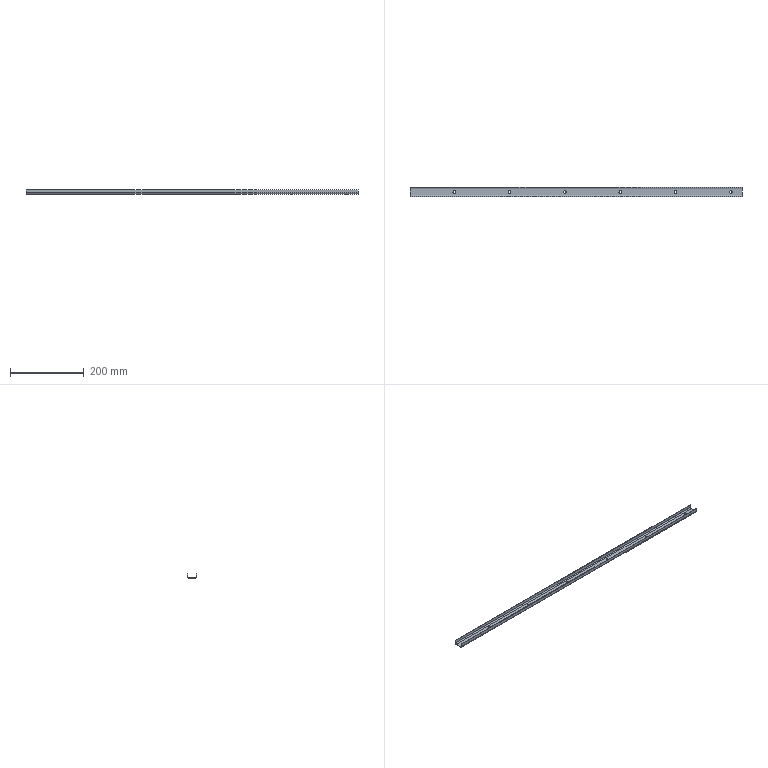Part | NX | features SKETCH 4, DATUM_CSYS 3, DATUM_PLANE 2, Flange 2, Base Tab 1, EXTRUDE 1 | 1 solid | 20 faces | box 900 x 25 x 12 mm | volume 46713 mm3 | plane 10 | cylinder 10 | commonest cylinder face diameters 7 x6 6 x2 8.4 x2
STEP:
#1=CARTESIAN_POINT('',(0.,20.8,0.));
#2=VERTEX_POINT('',#1);
#3=CARTESIAN_POINT('',(0.,4.2,0.));
#4=VERTEX_POINT('',#3);
#5=CARTESIAN_POINT('',(0.,25.,0.));
#6=DIRECTION('',(0.,-1.,0.));
#7=VECTOR('',#6,1000.);
#8=LINE('',#5,#7);
#9=EDGE_CURVE('',#2,#4,#8,.T.);
#10=ORIENTED_EDGE('',*,*,#9,.T.);
#11=CARTESIAN_POINT('',(0.,0.,4.2));
#12=VERTEX_POINT('',#11);
#13=CARTESIAN_POINT('',(0.,4.2,4.2));
#14=DIRECTION('',(-1.,0.,0.));
#15=DIRECTION('',(0.,0.,1.));
#16=AXIS2_PLACEMENT_3D('',#13,#14,#15);
#17=CIRCLE('',#16,4.2);
#18=EDGE_CURVE('',#4,#12,#17,.T.);
#19=ORIENTED_EDGE('',*,*,#18,.T.);
#20=CARTESIAN_POINT('',(0.,0.,12.));
#21=VERTEX_POINT('',#20);
#22=CARTESIAN_POINT('',(0.,0.,1.533));
#23=DIRECTION('',(0.,0.,1.));
#24=VECTOR('',#23,1000.);
#25=LINE('',#22,#24);
#26=EDGE_CURVE('',#12,#21,#25,.T.);
#27=ORIENTED_EDGE('',*,*,#26,.T.);
#28=CARTESIAN_POINT('',(0.,1.2,12.));
#29=VERTEX_POINT('',#28);
#30=CARTESIAN_POINT('',(0.,0.,12.));
#31=DIRECTION('',(0.,1.,0.));
#32=VECTOR('',#31,1000.);
#33=LINE('',#30,#32);
#34=EDGE_CURVE('',#21,#29,#33,.T.);
#35=ORIENTED_EDGE('',*,*,#34,.T.);
#36=CARTESIAN_POINT('',(0.,1.2,4.2));
#37=VERTEX_POINT('',#36);
#38=CARTESIAN_POINT('',(0.,1.2,1.533));
#39=DIRECTION('',(0.,0.,1.));
#40=VECTOR('',#39,1000.);
#41=LINE('',#38,#40);
#42=EDGE_CURVE('',#37,#29,#41,.T.);
#43=ORIENTED_EDGE('',*,*,#42,.F.);
#44=CARTESIAN_POINT('',(0.,4.2,1.2));
#45=VERTEX_POINT('',#44);
#46=CARTESIAN_POINT('',(0.,4.2,4.2));
#47=DIRECTION('',(-1.,0.,0.));
#48=DIRECTION('',(0.,0.,1.));
#49=AXIS2_PLACEMENT_3D('',#46,#47,#48);
#50=CIRCLE('',#49,3.);
#51=EDGE_CURVE('',#45,#37,#50,.T.);
#52=ORIENTED_EDGE('',*,*,#51,.F.);
#53=CARTESIAN_POINT('',(0.,20.8,1.2));
#54=VERTEX_POINT('',#53);
#55=CARTESIAN_POINT('',(0.,25.,1.2));
#56=DIRECTION('',(0.,-1.,0.));
#57=VECTOR('',#56,1000.);
#58=LINE('',#55,#57);
#59=EDGE_CURVE('',#54,#45,#58,.T.);
#60=ORIENTED_EDGE('',*,*,#59,.F.);
#61=CARTESIAN_POINT('',(0.,23.8,4.2));
#62=VERTEX_POINT('',#61);
#63=CARTESIAN_POINT('',(0.,20.8,4.2));
#64=DIRECTION('',(1.,0.,0.));
#65=DIRECTION('',(0.,0.,-1.));
#66=AXIS2_PLACEMENT_3D('',#63,#64,#65);
#67=CIRCLE('',#66,3.);
#68=EDGE_CURVE('',#62,#54,#67,.F.);
#69=ORIENTED_EDGE('',*,*,#68,.F.);
#70=CARTESIAN_POINT('',(0.,23.8,12.));
#71=VERTEX_POINT('',#70);
#72=CARTESIAN_POINT('',(0.,23.8,1.533));
#73=DIRECTION('',(0.,0.,1.));
#74=VECTOR('',#73,1000.);
#75=LINE('',#72,#74);
#76=EDGE_CURVE('',#62,#71,#75,.T.);
#77=ORIENTED_EDGE('',*,*,#76,.T.);
#78=CARTESIAN_POINT('',(0.,25.,12.));
#79=VERTEX_POINT('',#78);
#80=CARTESIAN_POINT('',(0.,25.,12.));
#81=DIRECTION('',(0.,-1.,0.));
#82=VECTOR('',#81,1000.);
#83=LINE('',#80,#82);
#84=EDGE_CURVE('',#79,#71,#83,.T.);
#85=ORIENTED_EDGE('',*,*,#84,.F.);
#86=CARTESIAN_POINT('',(0.,25.,4.2));
#87=VERTEX_POINT('',#86);
#88=CARTESIAN_POINT('',(0.,25.,1.533));
#89=DIRECTION('',(0.,0.,1.));
#90=VECTOR('',#89,1000.);
#91=LINE('',#88,#90);
#92=EDGE_CURVE('',#87,#79,#91,.T.);
#93=ORIENTED_EDGE('',*,*,#92,.F.);
#94=CARTESIAN_POINT('',(0.,20.8,4.2));
#95=DIRECTION('',(-1.,0.,0.));
#96=DIRECTION('',(0.,0.,1.));
#97=AXIS2_PLACEMENT_3D('',#94,#95,#96);
#98=CIRCLE('',#97,4.2);
#99=EDGE_CURVE('',#87,#2,#98,.T.);
#100=ORIENTED_EDGE('',*,*,#99,.T.);
#101=EDGE_LOOP('',(#10,#19,#27,#35,#43,#52,#60,#69,#77,#85,#93,#100));
#102=FACE_BOUND('',#101,.T.);
#103=CARTESIAN_POINT('',(0.,25.,1.2));
#104=DIRECTION('',(1.,0.,0.));
#105=DIRECTION('',(0.,1.,0.));
#106=AXIS2_PLACEMENT_3D('',#103,#104,#105);
#107=PLANE('',#106);
#108=ADVANCED_FACE('',(#102),#107,.F.);
#109=CARTESIAN_POINT('',(900.,4.2,1.2));
#110=VERTEX_POINT('',#109);
#111=CARTESIAN_POINT('',(900.,20.8,1.2));
#112=VERTEX_POINT('',#111);
#113=CARTESIAN_POINT('',(900.,0.,1.2));
#114=DIRECTION('',(0.,1.,0.));
#115=VECTOR('',#114,1000.);
#116=LINE('',#113,#115);
#117=EDGE_CURVE('',#110,#112,#116,.T.);
#118=ORIENTED_EDGE('',*,*,#117,.F.);
#119=CARTESIAN_POINT('',(900.,1.2,4.2));
#120=VERTEX_POINT('',#119);
#121=CARTESIAN_POINT('',(900.,4.2,4.2));
#122=DIRECTION('',(-1.,0.,0.));
#123=DIRECTION('',(0.,0.,1.));
#124=AXIS2_PLACEMENT_3D('',#121,#122,#123);
#125=CIRCLE('',#124,3.);
#126=EDGE_CURVE('',#120,#110,#125,.F.);
#127=ORIENTED_EDGE('',*,*,#126,.F.);
#128=CARTESIAN_POINT('',(900.,1.2,12.));
#129=VERTEX_POINT('',#128);
#130=CARTESIAN_POINT('',(900.,1.2,12.));
#131=DIRECTION('',(0.,0.,-1.));
#132=VECTOR('',#131,1000.);
#133=LINE('',#130,#132);
#134=EDGE_CURVE('',#129,#120,#133,.T.);
#135=ORIENTED_EDGE('',*,*,#134,.F.);
#136=CARTESIAN_POINT('',(900.,0.,12.));
#137=VERTEX_POINT('',#136);
#138=CARTESIAN_POINT('',(900.,0.,12.));
#139=DIRECTION('',(0.,1.,0.));
#140=VECTOR('',#139,1000.);
#141=LINE('',#138,#140);
#142=EDGE_CURVE('',#137,#129,#141,.T.);
#143=ORIENTED_EDGE('',*,*,#142,.F.);
#144=CARTESIAN_POINT('',(900.,0.,4.2));
#145=VERTEX_POINT('',#144);
#146=CARTESIAN_POINT('',(900.,0.,12.));
#147=DIRECTION('',(0.,0.,-1.));
#148=VECTOR('',#147,1000.);
#149=LINE('',#146,#148);
#150=EDGE_CURVE('',#137,#145,#149,.T.);
#151=ORIENTED_EDGE('',*,*,#150,.T.);
#152=CARTESIAN_POINT('',(900.,4.2,0.));
#153=VERTEX_POINT('',#152);
#154=CARTESIAN_POINT('',(900.,4.2,4.2));
#155=DIRECTION('',(1.,0.,0.));
#156=DIRECTION('',(0.,0.,1.));
#157=AXIS2_PLACEMENT_3D('',#154,#155,#156);
#158=CIRCLE('',#157,4.2);
#159=EDGE_CURVE('',#145,#153,#158,.T.);
#160=ORIENTED_EDGE('',*,*,#159,.T.);
#161=CARTESIAN_POINT('',(900.,20.8,0.));
#162=VERTEX_POINT('',#161);
#163=CARTESIAN_POINT('',(900.,0.,0.));
#164=DIRECTION('',(0.,1.,0.));
#165=VECTOR('',#164,1000.);
#166=LINE('',#163,#165);
#167=EDGE_CURVE('',#153,#162,#166,.T.);
#168=ORIENTED_EDGE('',*,*,#167,.T.);
#169=CARTESIAN_POINT('',(900.,25.,4.2));
#170=VERTEX_POINT('',#169);
#171=CARTESIAN_POINT('',(900.,20.8,4.2));
#172=DIRECTION('',(1.,0.,0.));
#173=DIRECTION('',(0.,0.,1.));
#174=AXIS2_PLACEMENT_3D('',#171,#172,#173);
#175=CIRCLE('',#174,4.2);
#176=EDGE_CURVE('',#162,#170,#175,.T.);
#177=ORIENTED_EDGE('',*,*,#176,.T.);
#178=CARTESIAN_POINT('',(900.,25.,12.));
#179=VERTEX_POINT('',#178);
#180=CARTESIAN_POINT('',(900.,25.,12.));
#181=DIRECTION('',(0.,0.,-1.));
#182=VECTOR('',#181,1000.);
#183=LINE('',#180,#182);
#184=EDGE_CURVE('',#179,#170,#183,.T.);
#185=ORIENTED_EDGE('',*,*,#184,.F.);
#186=CARTESIAN_POINT('',(900.,23.8,12.));
#187=VERTEX_POINT('',#186);
#188=CARTESIAN_POINT('',(900.,25.,12.));
#189=DIRECTION('',(0.,-1.,0.));
#190=VECTOR('',#189,1000.);
#191=LINE('',#188,#190);
#192=EDGE_CURVE('',#179,#187,#191,.T.);
#193=ORIENTED_EDGE('',*,*,#192,.T.);
#194=CARTESIAN_POINT('',(900.,23.8,4.2));
#195=VERTEX_POINT('',#194);
#196=CARTESIAN_POINT('',(900.,23.8,12.));
#197=DIRECTION('',(0.,0.,-1.));
#198=VECTOR('',#197,1000.);
#199=LINE('',#196,#198);
#200=EDGE_CURVE('',#187,#195,#199,.T.);
#201=ORIENTED_EDGE('',*,*,#200,.T.);
#202=CARTESIAN_POINT('',(900.,20.8,4.2));
#203=DIRECTION('',(1.,0.,0.));
#204=DIRECTION('',(0.,0.,-1.));
#205=AXIS2_PLACEMENT_3D('',#202,#203,#204);
#206=CIRCLE('',#205,3.);
#207=EDGE_CURVE('',#112,#195,#206,.T.);
#208=ORIENTED_EDGE('',*,*,#207,.F.);
#209=EDGE_LOOP('',(#118,#127,#135,#143,#151,#160,#168,#177,#185,#193,#201,#208));
#210=FACE_BOUND('',#209,.T.);
#211=CARTESIAN_POINT('',(900.,0.,1.2));
#212=DIRECTION('',(-1.,0.,0.));
#213=DIRECTION('',(0.,0.,1.));
#214=AXIS2_PLACEMENT_3D('',#211,#212,#213);
#215=PLANE('',#214);
#216=ADVANCED_FACE('',(#210),#215,.F.);
#217=CARTESIAN_POINT('',(123.5,12.5,0.));
#218=VERTEX_POINT('',#217);
#219=CARTESIAN_POINT('',(120.,12.5,0.));
#220=DIRECTION('',(0.,0.,1.));
#221=DIRECTION('',(1.,0.,0.));
#222=AXIS2_PLACEMENT_3D('',#219,#220,#221);
#223=CIRCLE('',#222,3.5);
#224=EDGE_CURVE('',#218,#218,#223,.T.);
#225=ORIENTED_EDGE('',*,*,#224,.T.);
#226=EDGE_LOOP('',(#225));
#227=FACE_BOUND('',#226,.T.);
#228=CARTESIAN_POINT('',(273.5,12.5,0.));
#229=VERTEX_POINT('',#228);
#230=CARTESIAN_POINT('',(270.,12.5,0.));
#231=DIRECTION('',(0.,0.,1.));
#232=DIRECTION('',(1.,0.,0.));
#233=AXIS2_PLACEMENT_3D('',#230,#231,#232);
#234=CIRCLE('',#233,3.5);
#235=EDGE_CURVE('',#229,#229,#234,.T.);
#236=ORIENTED_EDGE('',*,*,#235,.T.);
#237=EDGE_LOOP('',(#236));
#238=FACE_BOUND('',#237,.T.);
#239=CARTESIAN_POINT('',(423.5,12.5,0.));
#240=VERTEX_POINT('',#239);
#241=CARTESIAN_POINT('',(420.,12.5,0.));
#242=DIRECTION('',(0.,0.,1.));
#243=DIRECTION('',(1.,0.,0.));
#244=AXIS2_PLACEMENT_3D('',#241,#242,#243);
#245=CIRCLE('',#244,3.5);
#246=EDGE_CURVE('',#240,#240,#245,.T.);
#247=ORIENTED_EDGE('',*,*,#246,.T.);
#248=EDGE_LOOP('',(#247));
#249=FACE_BOUND('',#248,.T.);
#250=CARTESIAN_POINT('',(573.5,12.5,0.));
#251=VERTEX_POINT('',#250);
#252=CARTESIAN_POINT('',(570.,12.5,0.));
#253=DIRECTION('',(0.,0.,1.));
#254=DIRECTION('',(1.,0.,0.));
#255=AXIS2_PLACEMENT_3D('',#252,#253,#254);
#256=CIRCLE('',#255,3.5);
#257=EDGE_CURVE('',#251,#251,#256,.T.);
#258=ORIENTED_EDGE('',*,*,#257,.T.);
#259=EDGE_LOOP('',(#258));
#260=FACE_BOUND('',#259,.T.);
#261=CARTESIAN_POINT('',(723.5,12.5,0.));
#262=VERTEX_POINT('',#261);
#263=CARTESIAN_POINT('',(720.,12.5,0.));
#264=DIRECTION('',(0.,0.,1.));
#265=DIRECTION('',(1.,0.,0.));
#266=AXIS2_PLACEMENT_3D('',#263,#264,#265);
#267=CIRCLE('',#266,3.5);
#268=EDGE_CURVE('',#262,#262,#267,.T.);
#269=ORIENTED_EDGE('',*,*,#268,.T.);
#270=EDGE_LOOP('',(#269));
#271=FACE_BOUND('',#270,.T.);
#272=CARTESIAN_POINT('',(873.5,12.5,0.));
#273=VERTEX_POINT('',#272);
#274=CARTESIAN_POINT('',(870.,12.5,0.));
#275=DIRECTION('',(0.,0.,1.));
#276=DIRECTION('',(1.,0.,0.));
#277=AXIS2_PLACEMENT_3D('',#274,#275,#276);
#278=CIRCLE('',#277,3.5);
#279=EDGE_CURVE('',#273,#273,#278,.T.);
#280=ORIENTED_EDGE('',*,*,#279,.T.);
#281=EDGE_LOOP('',(#280));
#282=FACE_BOUND('',#281,.T.);
#283=ORIENTED_EDGE('',*,*,#167,.F.);
#284=CARTESIAN_POINT('',(900.,4.2,0.));
#285=DIRECTION('',(-1.,0.,0.));
#286=VECTOR('',#285,1000.);
#287=LINE('',#284,#286);
#288=EDGE_CURVE('',#153,#4,#287,.T.);
#289=ORIENTED_EDGE('',*,*,#288,.T.);
#290=ORIENTED_EDGE('',*,*,#9,.F.);
#291=CARTESIAN_POINT('',(0.,20.8,0.));
#292=DIRECTION('',(1.,0.,0.));
#293=VECTOR('',#292,1000.);
#294=LINE('',#291,#293);
#295=EDGE_CURVE('',#2,#162,#294,.T.);
#296=ORIENTED_EDGE('',*,*,#295,.T.);
#297=EDGE_LOOP('',(#283,#289,#290,#296));
#298=FACE_BOUND('',#297,.T.);
#299=CARTESIAN_POINT('',(0.,0.,0.));
#300=DIRECTION('',(0.,0.,1.));
#301=DIRECTION('',(1.,0.,0.));
#302=AXIS2_PLACEMENT_3D('',#299,#300,#301);
#303=PLANE('',#302);
#304=ADVANCED_FACE('',(#227,#238,#249,#260,#271,#282,#298),#303,.F.);
#305=CARTESIAN_POINT('',(116.5,12.5,1.2));
#306=VERTEX_POINT('',#305);
#307=CARTESIAN_POINT('',(120.,12.5,1.2));
#308=DIRECTION('',(0.,0.,1.));
#309=DIRECTION('',(-1.,0.,0.));
#310=AXIS2_PLACEMENT_3D('',#307,#308,#309);
#311=CIRCLE('',#310,3.5);
#312=EDGE_CURVE('',#306,#306,#311,.T.);
#313=ORIENTED_EDGE('',*,*,#312,.F.);
#314=EDGE_LOOP('',(#313));
#315=FACE_BOUND('',#314,.T.);
#316=CARTESIAN_POINT('',(266.5,12.5,1.2));
#317=VERTEX_POINT('',#316);
#318=CARTESIAN_POINT('',(270.,12.5,1.2));
#319=DIRECTION('',(0.,0.,1.));
#320=DIRECTION('',(-1.,0.,0.));
#321=AXIS2_PLACEMENT_3D('',#318,#319,#320);
#322=CIRCLE('',#321,3.5);
#323=EDGE_CURVE('',#317,#317,#322,.T.);
#324=ORIENTED_EDGE('',*,*,#323,.F.);
#325=EDGE_LOOP('',(#324));
#326=FACE_BOUND('',#325,.T.);
#327=CARTESIAN_POINT('',(416.5,12.5,1.2));
#328=VERTEX_POINT('',#327);
#329=CARTESIAN_POINT('',(420.,12.5,1.2));
#330=DIRECTION('',(0.,0.,1.));
#331=DIRECTION('',(-1.,0.,0.));
#332=AXIS2_PLACEMENT_3D('',#329,#330,#331);
#333=CIRCLE('',#332,3.5);
#334=EDGE_CURVE('',#328,#328,#333,.T.);
#335=ORIENTED_EDGE('',*,*,#334,.F.);
#336=EDGE_LOOP('',(#335));
#337=FACE_BOUND('',#336,.T.);
#338=CARTESIAN_POINT('',(566.5,12.5,1.2));
#339=VERTEX_POINT('',#338);
#340=CARTESIAN_POINT('',(570.,12.5,1.2));
#341=DIRECTION('',(0.,0.,1.));
#342=DIRECTION('',(-1.,0.,0.));
#343=AXIS2_PLACEMENT_3D('',#340,#341,#342);
#344=CIRCLE('',#343,3.5);
#345=EDGE_CURVE('',#339,#339,#344,.T.);
#346=ORIENTED_EDGE('',*,*,#345,.F.);
#347=EDGE_LOOP('',(#346));
#348=FACE_BOUND('',#347,.T.);
#349=CARTESIAN_POINT('',(716.5,12.5,1.2));
#350=VERTEX_POINT('',#349);
#351=CARTESIAN_POINT('',(720.,12.5,1.2));
#352=DIRECTION('',(0.,0.,1.));
#353=DIRECTION('',(-1.,0.,0.));
#354=AXIS2_PLACEMENT_3D('',#351,#352,#353);
#355=CIRCLE('',#354,3.5);
#356=EDGE_CURVE('',#350,#350,#355,.T.);
#357=ORIENTED_EDGE('',*,*,#356,.F.);
#358=EDGE_LOOP('',(#357));
#359=FACE_BOUND('',#358,.T.);
#360=CARTESIAN_POINT('',(866.5,12.5,1.2));
#361=VERTEX_POINT('',#360);
#362=CARTESIAN_POINT('',(870.,12.5,1.2));
#363=DIRECTION('',(0.,0.,1.));
#364=DIRECTION('',(-1.,0.,0.));
#365=AXIS2_PLACEMENT_3D('',#362,#363,#364);
#366=CIRCLE('',#365,3.5);
#367=EDGE_CURVE('',#361,#361,#366,.T.);
#368=ORIENTED_EDGE('',*,*,#367,.F.);
#369=EDGE_LOOP('',(#368));
#370=FACE_BOUND('',#369,.T.);
#371=CARTESIAN_POINT('',(900.,4.2,1.2));
#372=DIRECTION('',(-1.,0.,0.));
#373=VECTOR('',#372,1000.);
#374=LINE('',#371,#373);
#375=EDGE_CURVE('',#110,#45,#374,.T.);
#376=ORIENTED_EDGE('',*,*,#375,.F.);
#377=ORIENTED_EDGE('',*,*,#117,.T.);
#378=CARTESIAN_POINT('',(0.,20.8,1.2));
#379=DIRECTION('',(1.,0.,0.));
#380=VECTOR('',#379,1000.);
#381=LINE('',#378,#380);
#382=EDGE_CURVE('',#54,#112,#381,.T.);
#383=ORIENTED_EDGE('',*,*,#382,.F.);
#384=ORIENTED_EDGE('',*,*,#59,.T.);
#385=EDGE_LOOP('',(#376,#377,#383,#384));
#386=FACE_BOUND('',#385,.T.);
#387=CARTESIAN_POINT('',(0.,0.,1.2));
#388=DIRECTION('',(0.,0.,1.));
#389=DIRECTION('',(1.,0.,0.));
#390=AXIS2_PLACEMENT_3D('',#387,#388,#389);
#391=PLANE('',#390);
#392=ADVANCED_FACE('',(#315,#326,#337,#348,#359,#370,#386),#391,.T.);
#393=ORIENTED_EDGE('',*,*,#184,.T.);
#394=CARTESIAN_POINT('',(900.,25.,4.2));
#395=DIRECTION('',(-1.,0.,0.));
#396=VECTOR('',#395,1000.);
#397=LINE('',#394,#396);
#398=EDGE_CURVE('',#170,#87,#397,.T.);
#399=ORIENTED_EDGE('',*,*,#398,.T.);
#400=ORIENTED_EDGE('',*,*,#92,.T.);
#401=CARTESIAN_POINT('',(0.,25.,12.));
#402=DIRECTION('',(1.,0.,0.));
#403=VECTOR('',#402,1000.);
#404=LINE('',#401,#403);
#405=EDGE_CURVE('',#79,#179,#404,.T.);
#406=ORIENTED_EDGE('',*,*,#405,.T.);
#407=EDGE_LOOP('',(#393,#399,#400,#406));
#408=FACE_BOUND('',#407,.T.);
#409=CARTESIAN_POINT('',(0.,25.,0.));
#410=DIRECTION('',(0.,1.,0.));
#411=DIRECTION('',(-1.,0.,0.));
#412=AXIS2_PLACEMENT_3D('',#409,#410,#411);
#413=PLANE('',#412);
#414=ADVANCED_FACE('',(#408),#413,.T.);
#415=CARTESIAN_POINT('',(900.,23.8,4.2));
#416=DIRECTION('',(-1.,0.,0.));
#417=VECTOR('',#416,1000.);
#418=LINE('',#415,#417);
#419=EDGE_CURVE('',#195,#62,#418,.T.);
#420=ORIENTED_EDGE('',*,*,#419,.F.);
#421=ORIENTED_EDGE('',*,*,#200,.F.);
#422=CARTESIAN_POINT('',(0.,23.8,12.));
#423=DIRECTION('',(1.,0.,0.));
#424=VECTOR('',#423,1000.);
#425=LINE('',#422,#424);
#426=EDGE_CURVE('',#71,#187,#425,.T.);
#427=ORIENTED_EDGE('',*,*,#426,.F.);
#428=ORIENTED_EDGE('',*,*,#76,.F.);
#429=EDGE_LOOP('',(#420,#421,#427,#428));
#430=FACE_BOUND('',#429,.T.);
#431=CARTESIAN_POINT('',(0.,23.8,0.));
#432=DIRECTION('',(0.,1.,0.));
#433=DIRECTION('',(-1.,0.,0.));
#434=AXIS2_PLACEMENT_3D('',#431,#432,#433);
#435=PLANE('',#434);
#436=ADVANCED_FACE('',(#430),#435,.F.);
#437=ORIENTED_EDGE('',*,*,#426,.T.);
#438=ORIENTED_EDGE('',*,*,#192,.F.);
#439=ORIENTED_EDGE('',*,*,#405,.F.);
#440=ORIENTED_EDGE('',*,*,#84,.T.);
#441=EDGE_LOOP('',(#437,#438,#439,#440));
#442=FACE_BOUND('',#441,.T.);
#443=CARTESIAN_POINT('',(0.,25.,12.));
#444=DIRECTION('',(0.,0.,-1.));
#445=DIRECTION('',(0.,1.,0.));
#446=AXIS2_PLACEMENT_3D('',#443,#444,#445);
#447=PLANE('',#446);
#448=ADVANCED_FACE('',(#442),#447,.F.);
#449=ORIENTED_EDGE('',*,*,#295,.F.);
#450=ORIENTED_EDGE('',*,*,#99,.F.);
#451=ORIENTED_EDGE('',*,*,#398,.F.);
#452=ORIENTED_EDGE('',*,*,#176,.F.);
#453=EDGE_LOOP('',(#449,#450,#451,#452));
#454=FACE_BOUND('',#453,.T.);
#455=CARTESIAN_POINT('',(0.,20.8,4.2));
#456=DIRECTION('',(1.,0.,0.));
#457=DIRECTION('',(0.,0.,1.));
#458=AXIS2_PLACEMENT_3D('',#455,#456,#457);
#459=CYLINDRICAL_SURFACE('',#458,4.2);
#460=ADVANCED_FACE('',(#454),#459,.T.);
#461=ORIENTED_EDGE('',*,*,#382,.T.);
#462=ORIENTED_EDGE('',*,*,#207,.T.);
#463=ORIENTED_EDGE('',*,*,#419,.T.);
#464=ORIENTED_EDGE('',*,*,#68,.T.);
#465=EDGE_LOOP('',(#461,#462,#463,#464));
#466=FACE_BOUND('',#465,.T.);
#467=CARTESIAN_POINT('',(0.,20.8,4.2));
#468=DIRECTION('',(1.,0.,0.));
#469=DIRECTION('',(0.,0.,1.));
#470=AXIS2_PLACEMENT_3D('',#467,#468,#469);
#471=CYLINDRICAL_SURFACE('',#470,3.);
#472=ADVANCED_FACE('',(#466),#471,.F.);
#473=CARTESIAN_POINT('',(0.,0.,4.2));
#474=DIRECTION('',(1.,0.,0.));
#475=VECTOR('',#474,1000.);
#476=LINE('',#473,#475);
#477=EDGE_CURVE('',#12,#145,#476,.T.);
#478=ORIENTED_EDGE('',*,*,#477,.T.);
#479=ORIENTED_EDGE('',*,*,#150,.F.);
#480=CARTESIAN_POINT('',(0.,0.,12.));
#481=DIRECTION('',(1.,0.,0.));
#482=VECTOR('',#481,1000.);
#483=LINE('',#480,#482);
#484=EDGE_CURVE('',#21,#137,#483,.T.);
#485=ORIENTED_EDGE('',*,*,#484,.F.);
#486=ORIENTED_EDGE('',*,*,#26,.F.);
#487=EDGE_LOOP('',(#478,#479,#485,#486));
#488=FACE_BOUND('',#487,.T.);
#489=CARTESIAN_POINT('',(0.,0.,0.));
#490=DIRECTION('',(0.,1.,0.));
#491=DIRECTION('',(0.,0.,1.));
#492=AXIS2_PLACEMENT_3D('',#489,#490,#491);
#493=PLANE('',#492);
#494=ADVANCED_FACE('',(#488),#493,.F.);
#495=ORIENTED_EDGE('',*,*,#134,.T.);
#496=CARTESIAN_POINT('',(0.,1.2,4.2));
#497=DIRECTION('',(1.,0.,0.));
#498=VECTOR('',#497,1000.);
#499=LINE('',#496,#498);
#500=EDGE_CURVE('',#37,#120,#499,.T.);
#501=ORIENTED_EDGE('',*,*,#500,.F.);
#502=ORIENTED_EDGE('',*,*,#42,.T.);
#503=CARTESIAN_POINT('',(0.,1.2,12.));
#504=DIRECTION('',(1.,0.,0.));
#505=VECTOR('',#504,1000.);
#506=LINE('',#503,#505);
#507=EDGE_CURVE('',#29,#129,#506,.T.);
#508=ORIENTED_EDGE('',*,*,#507,.T.);
#509=EDGE_LOOP('',(#495,#501,#502,#508));
#510=FACE_BOUND('',#509,.T.);
#511=CARTESIAN_POINT('',(0.,1.2,0.));
#512=DIRECTION('',(0.,1.,0.));
#513=DIRECTION('',(0.,0.,1.));
#514=AXIS2_PLACEMENT_3D('',#511,#512,#513);
#515=PLANE('',#514);
#516=ADVANCED_FACE('',(#510),#515,.T.);
#517=ORIENTED_EDGE('',*,*,#507,.F.);
#518=ORIENTED_EDGE('',*,*,#34,.F.);
#519=ORIENTED_EDGE('',*,*,#484,.T.);
#520=ORIENTED_EDGE('',*,*,#142,.T.);
#521=EDGE_LOOP('',(#517,#518,#519,#520));
#522=FACE_BOUND('',#521,.T.);
#523=CARTESIAN_POINT('',(0.,0.,12.));
#524=DIRECTION('',(0.,0.,1.));
#525=DIRECTION('',(1.,0.,0.));
#526=AXIS2_PLACEMENT_3D('',#523,#524,#525);
#527=PLANE('',#526);
#528=ADVANCED_FACE('',(#522),#527,.T.);
#529=ORIENTED_EDGE('',*,*,#288,.F.);
#530=ORIENTED_EDGE('',*,*,#159,.F.);
#531=ORIENTED_EDGE('',*,*,#477,.F.);
#532=ORIENTED_EDGE('',*,*,#18,.F.);
#533=EDGE_LOOP('',(#529,#530,#531,#532));
#534=FACE_BOUND('',#533,.T.);
#535=CARTESIAN_POINT('',(900.,4.2,4.2));
#536=DIRECTION('',(-1.,0.,0.));
#537=DIRECTION('',(0.,0.,1.));
#538=AXIS2_PLACEMENT_3D('',#535,#536,#537);
#539=CYLINDRICAL_SURFACE('',#538,4.2);
#540=ADVANCED_FACE('',(#534),#539,.T.);
#541=ORIENTED_EDGE('',*,*,#375,.T.);
#542=ORIENTED_EDGE('',*,*,#51,.T.);
#543=ORIENTED_EDGE('',*,*,#500,.T.);
#544=ORIENTED_EDGE('',*,*,#126,.T.);
#545=EDGE_LOOP('',(#541,#542,#543,#544));
#546=FACE_BOUND('',#545,.T.);
#547=CARTESIAN_POINT('',(900.,4.2,4.2));
#548=DIRECTION('',(-1.,0.,0.));
#549=DIRECTION('',(0.,0.,1.));
#550=AXIS2_PLACEMENT_3D('',#547,#548,#549);
#551=CYLINDRICAL_SURFACE('',#550,3.);
#552=ADVANCED_FACE('',(#546),#551,.F.);
#553=ORIENTED_EDGE('',*,*,#367,.T.);
#554=EDGE_LOOP('',(#553));
#555=FACE_BOUND('',#554,.T.);
#556=ORIENTED_EDGE('',*,*,#279,.F.);
#557=EDGE_LOOP('',(#556));
#558=FACE_BOUND('',#557,.T.);
#559=CARTESIAN_POINT('',(870.,12.5,-28.8));
#560=DIRECTION('',(0.,0.,1.));
#561=DIRECTION('',(1.,0.,0.));
#562=AXIS2_PLACEMENT_3D('',#559,#560,#561);
#563=CYLINDRICAL_SURFACE('',#562,3.5);
#564=ADVANCED_FACE('',(#555,#558),#563,.F.);
#565=ORIENTED_EDGE('',*,*,#356,.T.);
#566=EDGE_LOOP('',(#565));
#567=FACE_BOUND('',#566,.T.);
#568=ORIENTED_EDGE('',*,*,#268,.F.);
#569=EDGE_LOOP('',(#568));
#570=FACE_BOUND('',#569,.T.);
#571=CARTESIAN_POINT('',(720.,12.5,-28.8));
#572=DIRECTION('',(0.,0.,1.));
#573=DIRECTION('',(1.,0.,0.));
#574=AXIS2_PLACEMENT_3D('',#571,#572,#573);
#575=CYLINDRICAL_SURFACE('',#574,3.5);
#576=ADVANCED_FACE('',(#567,#570),#575,.F.);
#577=ORIENTED_EDGE('',*,*,#345,.T.);
#578=EDGE_LOOP('',(#577));
#579=FACE_BOUND('',#578,.T.);
#580=ORIENTED_EDGE('',*,*,#257,.F.);
#581=EDGE_LOOP('',(#580));
#582=FACE_BOUND('',#581,.T.);
#583=CARTESIAN_POINT('',(570.,12.5,-28.8));
#584=DIRECTION('',(0.,0.,1.));
#585=DIRECTION('',(1.,0.,0.));
#586=AXIS2_PLACEMENT_3D('',#583,#584,#585);
#587=CYLINDRICAL_SURFACE('',#586,3.5);
#588=ADVANCED_FACE('',(#579,#582),#587,.F.);
#589=ORIENTED_EDGE('',*,*,#334,.T.);
#590=EDGE_LOOP('',(#589));
#591=FACE_BOUND('',#590,.T.);
#592=ORIENTED_EDGE('',*,*,#246,.F.);
#593=EDGE_LOOP('',(#592));
#594=FACE_BOUND('',#593,.T.);
#595=CARTESIAN_POINT('',(420.,12.5,-28.8));
#596=DIRECTION('',(0.,0.,1.));
#597=DIRECTION('',(1.,0.,0.));
#598=AXIS2_PLACEMENT_3D('',#595,#596,#597);
#599=CYLINDRICAL_SURFACE('',#598,3.5);
#600=ADVANCED_FACE('',(#591,#594),#599,.F.);
#601=ORIENTED_EDGE('',*,*,#323,.T.);
#602=EDGE_LOOP('',(#601));
#603=FACE_BOUND('',#602,.T.);
#604=ORIENTED_EDGE('',*,*,#235,.F.);
#605=EDGE_LOOP('',(#604));
#606=FACE_BOUND('',#605,.T.);
#607=CARTESIAN_POINT('',(270.,12.5,-28.8));
#608=DIRECTION('',(0.,0.,1.));
#609=DIRECTION('',(1.,0.,0.));
#610=AXIS2_PLACEMENT_3D('',#607,#608,#609);
#611=CYLINDRICAL_SURFACE('',#610,3.5);
#612=ADVANCED_FACE('',(#603,#606),#611,.F.);
#613=ORIENTED_EDGE('',*,*,#312,.T.);
#614=EDGE_LOOP('',(#613));
#615=FACE_BOUND('',#614,.T.);
#616=ORIENTED_EDGE('',*,*,#224,.F.);
#617=EDGE_LOOP('',(#616));
#618=FACE_BOUND('',#617,.T.);
#619=CARTESIAN_POINT('',(120.,12.5,-28.8));
#620=DIRECTION('',(0.,0.,1.));
#621=DIRECTION('',(1.,0.,0.));
#622=AXIS2_PLACEMENT_3D('',#619,#620,#621);
#623=CYLINDRICAL_SURFACE('',#622,3.5);
#624=ADVANCED_FACE('',(#615,#618),#623,.F.);
#625=CLOSED_SHELL('',(#108,#216,#304,#392,#414,#436,#448,#460,#472,#494,#516,#528,#540,#552,#564,#576,#588,#600,#612,#624));
#626=MANIFOLD_SOLID_BREP('',#625);
#627=(LENGTH_UNIT()NAMED_UNIT(*)SI_UNIT(.MILLI.,.METRE.));
#628=UNCERTAINTY_MEASURE_WITH_UNIT(LENGTH_MEASURE(0.00001),#627,'','');
#629=(NAMED_UNIT(*)PLANE_ANGLE_UNIT()SI_UNIT($,.RADIAN.));
#630=(NAMED_UNIT(*)SI_UNIT($,.STERADIAN.)SOLID_ANGLE_UNIT());
#631=(GEOMETRIC_REPRESENTATION_CONTEXT(3)GLOBAL_UNCERTAINTY_ASSIGNED_CONTEXT((#628))GLOBAL_UNIT_ASSIGNED_CONTEXT((#627,#629,#630))REPRESENTATION_CONTEXT('',''));
#632=ADVANCED_BREP_SHAPE_REPRESENTATION('',(#626),#631);